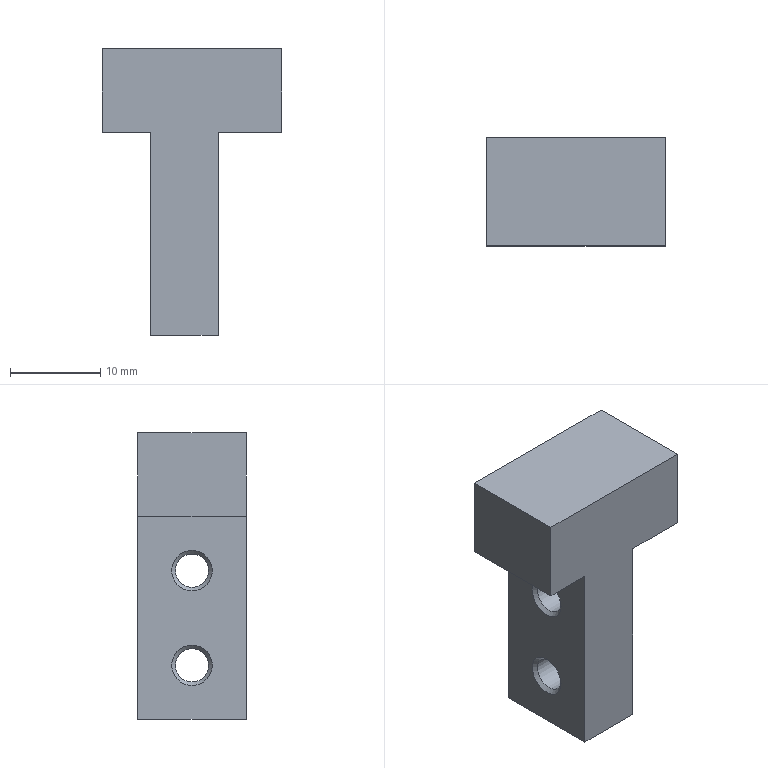Part | NX | features WGY01-16-6-2-001 2 | 1 solid | 16 faces | box 19.85 x 12 x 31.8 mm | volume 4076 mm3 | plane 10 | cone 4 | cylinder 2 | commonest cylinder face diameters 3.688 x2
STEP:
#1=CARTESIAN_POINT('',(88.248,-40.45,-26.));
#2=VERTEX_POINT('',#1);
#3=CARTESIAN_POINT('',(88.248,-42.7,-26.));
#4=DIRECTION('',(-1.,0.,0.));
#5=DIRECTION('',(0.,1.,0.));
#6=AXIS2_PLACEMENT_3D('',#3,#4,#5);
#7=CIRCLE('',#6,2.25);
#8=EDGE_CURVE('',#2,#2,#7,.F.);
#9=ORIENTED_EDGE('',*,*,#8,.T.);
#10=EDGE_LOOP('',(#9));
#11=FACE_BOUND('',#10,.T.);
#12=CARTESIAN_POINT('',(87.843,-40.856,-26.));
#13=VERTEX_POINT('',#12);
#14=CARTESIAN_POINT('',(87.843,-42.7,-26.));
#15=DIRECTION('',(-1.,0.,0.));
#16=DIRECTION('',(0.,1.,0.));
#17=AXIS2_PLACEMENT_3D('',#14,#15,#16);
#18=CIRCLE('',#17,1.844);
#19=EDGE_CURVE('',#13,#13,#18,.F.);
#20=ORIENTED_EDGE('',*,*,#19,.F.);
#21=EDGE_LOOP('',(#20));
#22=FACE_BOUND('',#21,.T.);
#23=CARTESIAN_POINT('',(87.843,-42.7,-26.));
#24=DIRECTION('',(1.,0.,0.));
#25=DIRECTION('',(0.,-1.,0.));
#26=AXIS2_PLACEMENT_3D('',#23,#24,#25);
#27=CONICAL_SURFACE('',#26,1.844,0.7854);
#28=ADVANCED_FACE('',(#11,#22),#27,.F.);
#29=ORIENTED_EDGE('',*,*,#19,.T.);
#30=EDGE_LOOP('',(#29));
#31=FACE_BOUND('',#30,.T.);
#32=CARTESIAN_POINT('',(81.154,-44.544,-26.));
#33=VERTEX_POINT('',#32);
#34=CARTESIAN_POINT('',(81.154,-42.7,-26.));
#35=DIRECTION('',(1.,0.,0.));
#36=DIRECTION('',(0.,-1.,0.));
#37=AXIS2_PLACEMENT_3D('',#34,#35,#36);
#38=CIRCLE('',#37,1.844);
#39=EDGE_CURVE('',#33,#33,#38,.T.);
#40=ORIENTED_EDGE('',*,*,#39,.F.);
#41=EDGE_LOOP('',(#40));
#42=FACE_BOUND('',#41,.T.);
#43=CARTESIAN_POINT('',(88.248,-42.7,-26.));
#44=DIRECTION('',(1.,0.,0.));
#45=DIRECTION('',(0.,-1.,0.));
#46=AXIS2_PLACEMENT_3D('',#43,#44,#45);
#47=CYLINDRICAL_SURFACE('',#46,1.844);
#48=ADVANCED_FACE('',(#31,#42),#47,.F.);
#49=CARTESIAN_POINT('',(80.748,-44.95,-26.));
#50=VERTEX_POINT('',#49);
#51=CARTESIAN_POINT('',(80.748,-42.7,-26.));
#52=DIRECTION('',(1.,0.,0.));
#53=DIRECTION('',(0.,-1.,0.));
#54=AXIS2_PLACEMENT_3D('',#51,#52,#53);
#55=CIRCLE('',#54,2.25);
#56=EDGE_CURVE('',#50,#50,#55,.T.);
#57=ORIENTED_EDGE('',*,*,#56,.F.);
#58=EDGE_LOOP('',(#57));
#59=FACE_BOUND('',#58,.T.);
#60=ORIENTED_EDGE('',*,*,#39,.T.);
#61=EDGE_LOOP('',(#60));
#62=FACE_BOUND('',#61,.T.);
#63=CARTESIAN_POINT('',(80.748,-42.7,-26.));
#64=DIRECTION('',(-1.,0.,0.));
#65=DIRECTION('',(0.,1.,0.));
#66=AXIS2_PLACEMENT_3D('',#63,#64,#65);
#67=CONICAL_SURFACE('',#66,2.25,0.7854);
#68=ADVANCED_FACE('',(#59,#62),#67,.F.);
#69=CARTESIAN_POINT('',(88.248,-40.45,-36.5));
#70=VERTEX_POINT('',#69);
#71=CARTESIAN_POINT('',(88.248,-42.7,-36.5));
#72=DIRECTION('',(-1.,0.,0.));
#73=DIRECTION('',(0.,1.,0.));
#74=AXIS2_PLACEMENT_3D('',#71,#72,#73);
#75=CIRCLE('',#74,2.25);
#76=EDGE_CURVE('',#70,#70,#75,.F.);
#77=ORIENTED_EDGE('',*,*,#76,.T.);
#78=EDGE_LOOP('',(#77));
#79=FACE_BOUND('',#78,.T.);
#80=CARTESIAN_POINT('',(87.843,-40.856,-36.5));
#81=VERTEX_POINT('',#80);
#82=CARTESIAN_POINT('',(87.843,-42.7,-36.5));
#83=DIRECTION('',(-1.,0.,0.));
#84=DIRECTION('',(0.,1.,0.));
#85=AXIS2_PLACEMENT_3D('',#82,#83,#84);
#86=CIRCLE('',#85,1.844);
#87=EDGE_CURVE('',#81,#81,#86,.F.);
#88=ORIENTED_EDGE('',*,*,#87,.F.);
#89=EDGE_LOOP('',(#88));
#90=FACE_BOUND('',#89,.T.);
#91=CARTESIAN_POINT('',(87.843,-42.7,-36.5));
#92=DIRECTION('',(1.,0.,0.));
#93=DIRECTION('',(0.,-1.,0.));
#94=AXIS2_PLACEMENT_3D('',#91,#92,#93);
#95=CONICAL_SURFACE('',#94,1.844,0.7854);
#96=ADVANCED_FACE('',(#79,#90),#95,.F.);
#97=ORIENTED_EDGE('',*,*,#87,.T.);
#98=EDGE_LOOP('',(#97));
#99=FACE_BOUND('',#98,.T.);
#100=CARTESIAN_POINT('',(81.154,-44.544,-36.5));
#101=VERTEX_POINT('',#100);
#102=CARTESIAN_POINT('',(81.154,-42.7,-36.5));
#103=DIRECTION('',(1.,0.,0.));
#104=DIRECTION('',(0.,-1.,0.));
#105=AXIS2_PLACEMENT_3D('',#102,#103,#104);
#106=CIRCLE('',#105,1.844);
#107=EDGE_CURVE('',#101,#101,#106,.T.);
#108=ORIENTED_EDGE('',*,*,#107,.F.);
#109=EDGE_LOOP('',(#108));
#110=FACE_BOUND('',#109,.T.);
#111=CARTESIAN_POINT('',(88.248,-42.7,-36.5));
#112=DIRECTION('',(1.,0.,0.));
#113=DIRECTION('',(0.,-1.,0.));
#114=AXIS2_PLACEMENT_3D('',#111,#112,#113);
#115=CYLINDRICAL_SURFACE('',#114,1.844);
#116=ADVANCED_FACE('',(#99,#110),#115,.F.);
#117=CARTESIAN_POINT('',(80.748,-44.95,-36.5));
#118=VERTEX_POINT('',#117);
#119=CARTESIAN_POINT('',(80.748,-42.7,-36.5));
#120=DIRECTION('',(1.,0.,0.));
#121=DIRECTION('',(0.,-1.,0.));
#122=AXIS2_PLACEMENT_3D('',#119,#120,#121);
#123=CIRCLE('',#122,2.25);
#124=EDGE_CURVE('',#118,#118,#123,.T.);
#125=ORIENTED_EDGE('',*,*,#124,.F.);
#126=EDGE_LOOP('',(#125));
#127=FACE_BOUND('',#126,.T.);
#128=ORIENTED_EDGE('',*,*,#107,.T.);
#129=EDGE_LOOP('',(#128));
#130=FACE_BOUND('',#129,.T.);
#131=CARTESIAN_POINT('',(80.748,-42.7,-36.5));
#132=DIRECTION('',(-1.,0.,0.));
#133=DIRECTION('',(0.,1.,0.));
#134=AXIS2_PLACEMENT_3D('',#131,#132,#133);
#135=CONICAL_SURFACE('',#134,2.25,0.7854);
#136=ADVANCED_FACE('',(#127,#130),#135,.F.);
#137=CARTESIAN_POINT('',(75.423,-36.7,-10.7));
#138=VERTEX_POINT('',#137);
#139=CARTESIAN_POINT('',(75.423,-36.7,-20.));
#140=VERTEX_POINT('',#139);
#141=CARTESIAN_POINT('',(75.423,-36.7,-20.));
#142=DIRECTION('',(0.,0.,1.));
#143=VECTOR('',#142,1000.);
#144=LINE('',#141,#143);
#145=EDGE_CURVE('',#138,#140,#144,.F.);
#146=ORIENTED_EDGE('',*,*,#145,.T.);
#147=CARTESIAN_POINT('',(75.423,-48.7,-20.));
#148=VERTEX_POINT('',#147);
#149=CARTESIAN_POINT('',(75.423,-48.7,-20.));
#150=DIRECTION('',(0.,1.,0.));
#151=VECTOR('',#150,1000.);
#152=LINE('',#149,#151);
#153=EDGE_CURVE('',#140,#148,#152,.F.);
#154=ORIENTED_EDGE('',*,*,#153,.T.);
#155=CARTESIAN_POINT('',(75.423,-48.7,-10.7));
#156=VERTEX_POINT('',#155);
#157=CARTESIAN_POINT('',(75.423,-48.7,-20.));
#158=DIRECTION('',(0.,0.,1.));
#159=VECTOR('',#158,1000.);
#160=LINE('',#157,#159);
#161=EDGE_CURVE('',#156,#148,#160,.F.);
#162=ORIENTED_EDGE('',*,*,#161,.F.);
#163=CARTESIAN_POINT('',(75.423,-48.7,-10.7));
#164=DIRECTION('',(0.,1.,0.));
#165=VECTOR('',#164,1000.);
#166=LINE('',#163,#165);
#167=EDGE_CURVE('',#138,#156,#166,.F.);
#168=ORIENTED_EDGE('',*,*,#167,.F.);
#169=EDGE_LOOP('',(#146,#154,#162,#168));
#170=FACE_BOUND('',#169,.T.);
#171=CARTESIAN_POINT('',(75.423,-48.7,-20.));
#172=DIRECTION('',(1.,0.,0.));
#173=DIRECTION('',(0.,-1.,0.));
#174=AXIS2_PLACEMENT_3D('',#171,#172,#173);
#175=PLANE('',#174);
#176=ADVANCED_FACE('',(#170),#175,.F.);
#177=CARTESIAN_POINT('',(95.273,-36.7,-10.7));
#178=VERTEX_POINT('',#177);
#179=CARTESIAN_POINT('',(75.423,-36.7,-10.7));
#180=DIRECTION('',(1.,0.,0.));
#181=VECTOR('',#180,1000.);
#182=LINE('',#179,#181);
#183=EDGE_CURVE('',#178,#138,#182,.F.);
#184=ORIENTED_EDGE('',*,*,#183,.T.);
#185=ORIENTED_EDGE('',*,*,#167,.T.);
#186=CARTESIAN_POINT('',(95.273,-48.7,-10.7));
#187=VERTEX_POINT('',#186);
#188=CARTESIAN_POINT('',(75.423,-48.7,-10.7));
#189=DIRECTION('',(1.,0.,0.));
#190=VECTOR('',#189,1000.);
#191=LINE('',#188,#190);
#192=EDGE_CURVE('',#187,#156,#191,.F.);
#193=ORIENTED_EDGE('',*,*,#192,.F.);
#194=CARTESIAN_POINT('',(95.273,-48.7,-10.7));
#195=DIRECTION('',(0.,-1.,0.));
#196=VECTOR('',#195,1000.);
#197=LINE('',#194,#196);
#198=EDGE_CURVE('',#178,#187,#197,.T.);
#199=ORIENTED_EDGE('',*,*,#198,.F.);
#200=EDGE_LOOP('',(#184,#185,#193,#199));
#201=FACE_BOUND('',#200,.T.);
#202=CARTESIAN_POINT('',(75.423,-48.7,-10.7));
#203=DIRECTION('',(0.,0.,-1.));
#204=DIRECTION('',(1.,0.,0.));
#205=AXIS2_PLACEMENT_3D('',#202,#203,#204);
#206=PLANE('',#205);
#207=ADVANCED_FACE('',(#201),#206,.F.);
#208=CARTESIAN_POINT('',(95.273,-36.7,-20.));
#209=VERTEX_POINT('',#208);
#210=CARTESIAN_POINT('',(95.273,-36.7,-10.7));
#211=DIRECTION('',(0.,0.,1.));
#212=VECTOR('',#211,1000.);
#213=LINE('',#210,#212);
#214=EDGE_CURVE('',#209,#178,#213,.T.);
#215=ORIENTED_EDGE('',*,*,#214,.T.);
#216=ORIENTED_EDGE('',*,*,#198,.T.);
#217=CARTESIAN_POINT('',(95.273,-48.7,-20.));
#218=VERTEX_POINT('',#217);
#219=CARTESIAN_POINT('',(95.273,-48.7,-10.7));
#220=DIRECTION('',(0.,0.,1.));
#221=VECTOR('',#220,1000.);
#222=LINE('',#219,#221);
#223=EDGE_CURVE('',#218,#187,#222,.T.);
#224=ORIENTED_EDGE('',*,*,#223,.F.);
#225=CARTESIAN_POINT('',(95.273,-48.7,-20.));
#226=DIRECTION('',(0.,-1.,0.));
#227=VECTOR('',#226,1000.);
#228=LINE('',#225,#227);
#229=EDGE_CURVE('',#209,#218,#228,.T.);
#230=ORIENTED_EDGE('',*,*,#229,.F.);
#231=EDGE_LOOP('',(#215,#216,#224,#230));
#232=FACE_BOUND('',#231,.T.);
#233=CARTESIAN_POINT('',(95.273,-48.7,-10.7));
#234=DIRECTION('',(-1.,0.,0.));
#235=DIRECTION('',(0.,1.,0.));
#236=AXIS2_PLACEMENT_3D('',#233,#234,#235);
#237=PLANE('',#236);
#238=ADVANCED_FACE('',(#232),#237,.F.);
#239=CARTESIAN_POINT('',(88.248,-36.7,-20.));
#240=VERTEX_POINT('',#239);
#241=CARTESIAN_POINT('',(99.273,-36.7,-20.));
#242=DIRECTION('',(-1.,0.,0.));
#243=VECTOR('',#242,1000.);
#244=LINE('',#241,#243);
#245=EDGE_CURVE('',#240,#209,#244,.F.);
#246=ORIENTED_EDGE('',*,*,#245,.T.);
#247=ORIENTED_EDGE('',*,*,#229,.T.);
#248=CARTESIAN_POINT('',(88.248,-48.7,-20.));
#249=VERTEX_POINT('',#248);
#250=CARTESIAN_POINT('',(99.273,-48.7,-20.));
#251=DIRECTION('',(-1.,0.,0.));
#252=VECTOR('',#251,1000.);
#253=LINE('',#250,#252);
#254=EDGE_CURVE('',#249,#218,#253,.F.);
#255=ORIENTED_EDGE('',*,*,#254,.F.);
#256=CARTESIAN_POINT('',(88.248,-48.7,-20.));
#257=DIRECTION('',(0.,1.,0.));
#258=VECTOR('',#257,1000.);
#259=LINE('',#256,#258);
#260=EDGE_CURVE('',#240,#249,#259,.F.);
#261=ORIENTED_EDGE('',*,*,#260,.F.);
#262=EDGE_LOOP('',(#246,#247,#255,#261));
#263=FACE_BOUND('',#262,.T.);
#264=CARTESIAN_POINT('',(99.273,-48.7,-20.));
#265=DIRECTION('',(0.,0.,1.));
#266=DIRECTION('',(-1.,0.,0.));
#267=AXIS2_PLACEMENT_3D('',#264,#265,#266);
#268=PLANE('',#267);
#269=ADVANCED_FACE('',(#263),#268,.F.);
#270=ORIENTED_EDGE('',*,*,#8,.F.);
#271=EDGE_LOOP('',(#270));
#272=FACE_BOUND('',#271,.T.);
#273=ORIENTED_EDGE('',*,*,#76,.F.);
#274=EDGE_LOOP('',(#273));
#275=FACE_BOUND('',#274,.T.);
#276=CARTESIAN_POINT('',(88.248,-36.7,-42.5));
#277=VERTEX_POINT('',#276);
#278=CARTESIAN_POINT('',(88.248,-36.7,-20.));
#279=DIRECTION('',(0.,0.,-1.));
#280=VECTOR('',#279,1000.);
#281=LINE('',#278,#280);
#282=EDGE_CURVE('',#277,#240,#281,.F.);
#283=ORIENTED_EDGE('',*,*,#282,.T.);
#284=ORIENTED_EDGE('',*,*,#260,.T.);
#285=CARTESIAN_POINT('',(88.248,-48.7,-42.5));
#286=VERTEX_POINT('',#285);
#287=CARTESIAN_POINT('',(88.248,-48.7,-20.));
#288=DIRECTION('',(0.,0.,-1.));
#289=VECTOR('',#288,1000.);
#290=LINE('',#287,#289);
#291=EDGE_CURVE('',#286,#249,#290,.F.);
#292=ORIENTED_EDGE('',*,*,#291,.F.);
#293=CARTESIAN_POINT('',(88.248,-48.7,-42.5));
#294=DIRECTION('',(0.,1.,0.));
#295=VECTOR('',#294,1000.);
#296=LINE('',#293,#295);
#297=EDGE_CURVE('',#277,#286,#296,.F.);
#298=ORIENTED_EDGE('',*,*,#297,.F.);
#299=EDGE_LOOP('',(#283,#284,#292,#298));
#300=FACE_BOUND('',#299,.T.);
#301=CARTESIAN_POINT('',(88.248,-48.7,-20.));
#302=DIRECTION('',(-1.,0.,0.));
#303=DIRECTION('',(0.,1.,0.));
#304=AXIS2_PLACEMENT_3D('',#301,#302,#303);
#305=PLANE('',#304);
#306=ADVANCED_FACE('',(#272,#275,#300),#305,.F.);
#307=CARTESIAN_POINT('',(80.748,-36.7,-42.5));
#308=VERTEX_POINT('',#307);
#309=CARTESIAN_POINT('',(88.248,-36.7,-42.5));
#310=DIRECTION('',(-1.,0.,0.));
#311=VECTOR('',#310,1000.);
#312=LINE('',#309,#311);
#313=EDGE_CURVE('',#308,#277,#312,.F.);
#314=ORIENTED_EDGE('',*,*,#313,.T.);
#315=ORIENTED_EDGE('',*,*,#297,.T.);
#316=CARTESIAN_POINT('',(80.748,-48.7,-42.5));
#317=VERTEX_POINT('',#316);
#318=CARTESIAN_POINT('',(88.248,-48.7,-42.5));
#319=DIRECTION('',(-1.,0.,0.));
#320=VECTOR('',#319,1000.);
#321=LINE('',#318,#320);
#322=EDGE_CURVE('',#317,#286,#321,.F.);
#323=ORIENTED_EDGE('',*,*,#322,.F.);
#324=CARTESIAN_POINT('',(80.748,-48.7,-42.5));
#325=DIRECTION('',(0.,1.,0.));
#326=VECTOR('',#325,1000.);
#327=LINE('',#324,#326);
#328=EDGE_CURVE('',#308,#317,#327,.F.);
#329=ORIENTED_EDGE('',*,*,#328,.F.);
#330=EDGE_LOOP('',(#314,#315,#323,#329));
#331=FACE_BOUND('',#330,.T.);
#332=CARTESIAN_POINT('',(88.248,-48.7,-42.5));
#333=DIRECTION('',(0.,0.,1.));
#334=DIRECTION('',(-1.,0.,0.));
#335=AXIS2_PLACEMENT_3D('',#332,#333,#334);
#336=PLANE('',#335);
#337=ADVANCED_FACE('',(#331),#336,.F.);
#338=ORIENTED_EDGE('',*,*,#56,.T.);
#339=EDGE_LOOP('',(#338));
#340=FACE_BOUND('',#339,.T.);
#341=ORIENTED_EDGE('',*,*,#124,.T.);
#342=EDGE_LOOP('',(#341));
#343=FACE_BOUND('',#342,.T.);
#344=CARTESIAN_POINT('',(80.748,-36.7,-20.));
#345=VERTEX_POINT('',#344);
#346=CARTESIAN_POINT('',(80.748,-36.7,-42.5));
#347=DIRECTION('',(0.,0.,1.));
#348=VECTOR('',#347,1000.);
#349=LINE('',#346,#348);
#350=EDGE_CURVE('',#345,#308,#349,.F.);
#351=ORIENTED_EDGE('',*,*,#350,.T.);
#352=ORIENTED_EDGE('',*,*,#328,.T.);
#353=CARTESIAN_POINT('',(80.748,-48.7,-20.));
#354=VERTEX_POINT('',#353);
#355=CARTESIAN_POINT('',(80.748,-48.7,-42.5));
#356=DIRECTION('',(0.,0.,1.));
#357=VECTOR('',#356,1000.);
#358=LINE('',#355,#357);
#359=EDGE_CURVE('',#354,#317,#358,.F.);
#360=ORIENTED_EDGE('',*,*,#359,.F.);
#361=CARTESIAN_POINT('',(80.748,-48.7,-20.));
#362=DIRECTION('',(0.,1.,0.));
#363=VECTOR('',#362,1000.);
#364=LINE('',#361,#363);
#365=EDGE_CURVE('',#345,#354,#364,.F.);
#366=ORIENTED_EDGE('',*,*,#365,.F.);
#367=EDGE_LOOP('',(#351,#352,#360,#366));
#368=FACE_BOUND('',#367,.T.);
#369=CARTESIAN_POINT('',(80.748,-48.7,-42.5));
#370=DIRECTION('',(1.,0.,0.));
#371=DIRECTION('',(0.,-1.,0.));
#372=AXIS2_PLACEMENT_3D('',#369,#370,#371);
#373=PLANE('',#372);
#374=ADVANCED_FACE('',(#340,#343,#368),#373,.F.);
#375=CARTESIAN_POINT('',(80.748,-36.7,-20.));
#376=DIRECTION('',(-1.,0.,0.));
#377=VECTOR('',#376,1000.);
#378=LINE('',#375,#377);
#379=EDGE_CURVE('',#140,#345,#378,.F.);
#380=ORIENTED_EDGE('',*,*,#379,.T.);
#381=ORIENTED_EDGE('',*,*,#365,.T.);
#382=CARTESIAN_POINT('',(80.748,-48.7,-20.));
#383=DIRECTION('',(-1.,0.,0.));
#384=VECTOR('',#383,1000.);
#385=LINE('',#382,#384);
#386=EDGE_CURVE('',#148,#354,#385,.F.);
#387=ORIENTED_EDGE('',*,*,#386,.F.);
#388=ORIENTED_EDGE('',*,*,#153,.F.);
#389=EDGE_LOOP('',(#380,#381,#387,#388));
#390=FACE_BOUND('',#389,.T.);
#391=CARTESIAN_POINT('',(80.748,-48.7,-20.));
#392=DIRECTION('',(0.,0.,1.));
#393=DIRECTION('',(-1.,0.,0.));
#394=AXIS2_PLACEMENT_3D('',#391,#392,#393);
#395=PLANE('',#394);
#396=ADVANCED_FACE('',(#390),#395,.F.);
#397=ORIENTED_EDGE('',*,*,#161,.T.);
#398=ORIENTED_EDGE('',*,*,#386,.T.);
#399=ORIENTED_EDGE('',*,*,#359,.T.);
#400=ORIENTED_EDGE('',*,*,#322,.T.);
#401=ORIENTED_EDGE('',*,*,#291,.T.);
#402=ORIENTED_EDGE('',*,*,#254,.T.);
#403=ORIENTED_EDGE('',*,*,#223,.T.);
#404=ORIENTED_EDGE('',*,*,#192,.T.);
#405=EDGE_LOOP('',(#397,#398,#399,#400,#401,#402,#403,#404));
#406=FACE_BOUND('',#405,.T.);
#407=CARTESIAN_POINT('',(84.498,-48.7,-16.55));
#408=DIRECTION('',(0.,-1.,0.));
#409=DIRECTION('',(-1.,0.,0.));
#410=AXIS2_PLACEMENT_3D('',#407,#408,#409);
#411=PLANE('',#410);
#412=ADVANCED_FACE('',(#406),#411,.T.);
#413=ORIENTED_EDGE('',*,*,#145,.F.);
#414=ORIENTED_EDGE('',*,*,#183,.F.);
#415=ORIENTED_EDGE('',*,*,#214,.F.);
#416=ORIENTED_EDGE('',*,*,#245,.F.);
#417=ORIENTED_EDGE('',*,*,#282,.F.);
#418=ORIENTED_EDGE('',*,*,#313,.F.);
#419=ORIENTED_EDGE('',*,*,#350,.F.);
#420=ORIENTED_EDGE('',*,*,#379,.F.);
#421=EDGE_LOOP('',(#413,#414,#415,#416,#417,#418,#419,#420));
#422=FACE_BOUND('',#421,.T.);
#423=CARTESIAN_POINT('',(84.498,-36.7,-16.55));
#424=DIRECTION('',(0.,-1.,0.));
#425=DIRECTION('',(-1.,0.,0.));
#426=AXIS2_PLACEMENT_3D('',#423,#424,#425);
#427=PLANE('',#426);
#428=ADVANCED_FACE('',(#422),#427,.F.);
#429=CLOSED_SHELL('',(#28,#48,#68,#96,#116,#136,#176,#207,#238,#269,#306,#337,#374,#396,#412,#428));
#430=MANIFOLD_SOLID_BREP('',#429);
#431=(LENGTH_UNIT()NAMED_UNIT(*)SI_UNIT(.MILLI.,.METRE.));
#432=UNCERTAINTY_MEASURE_WITH_UNIT(LENGTH_MEASURE(0.00001),#431,'','');
#433=(NAMED_UNIT(*)PLANE_ANGLE_UNIT()SI_UNIT($,.RADIAN.));
#434=(NAMED_UNIT(*)SI_UNIT($,.STERADIAN.)SOLID_ANGLE_UNIT());
#435=(GEOMETRIC_REPRESENTATION_CONTEXT(3)GLOBAL_UNCERTAINTY_ASSIGNED_CONTEXT((#432))GLOBAL_UNIT_ASSIGNED_CONTEXT((#431,#433,#434))REPRESENTATION_CONTEXT('',''));
#436=ADVANCED_BREP_SHAPE_REPRESENTATION('',(#430),#435);